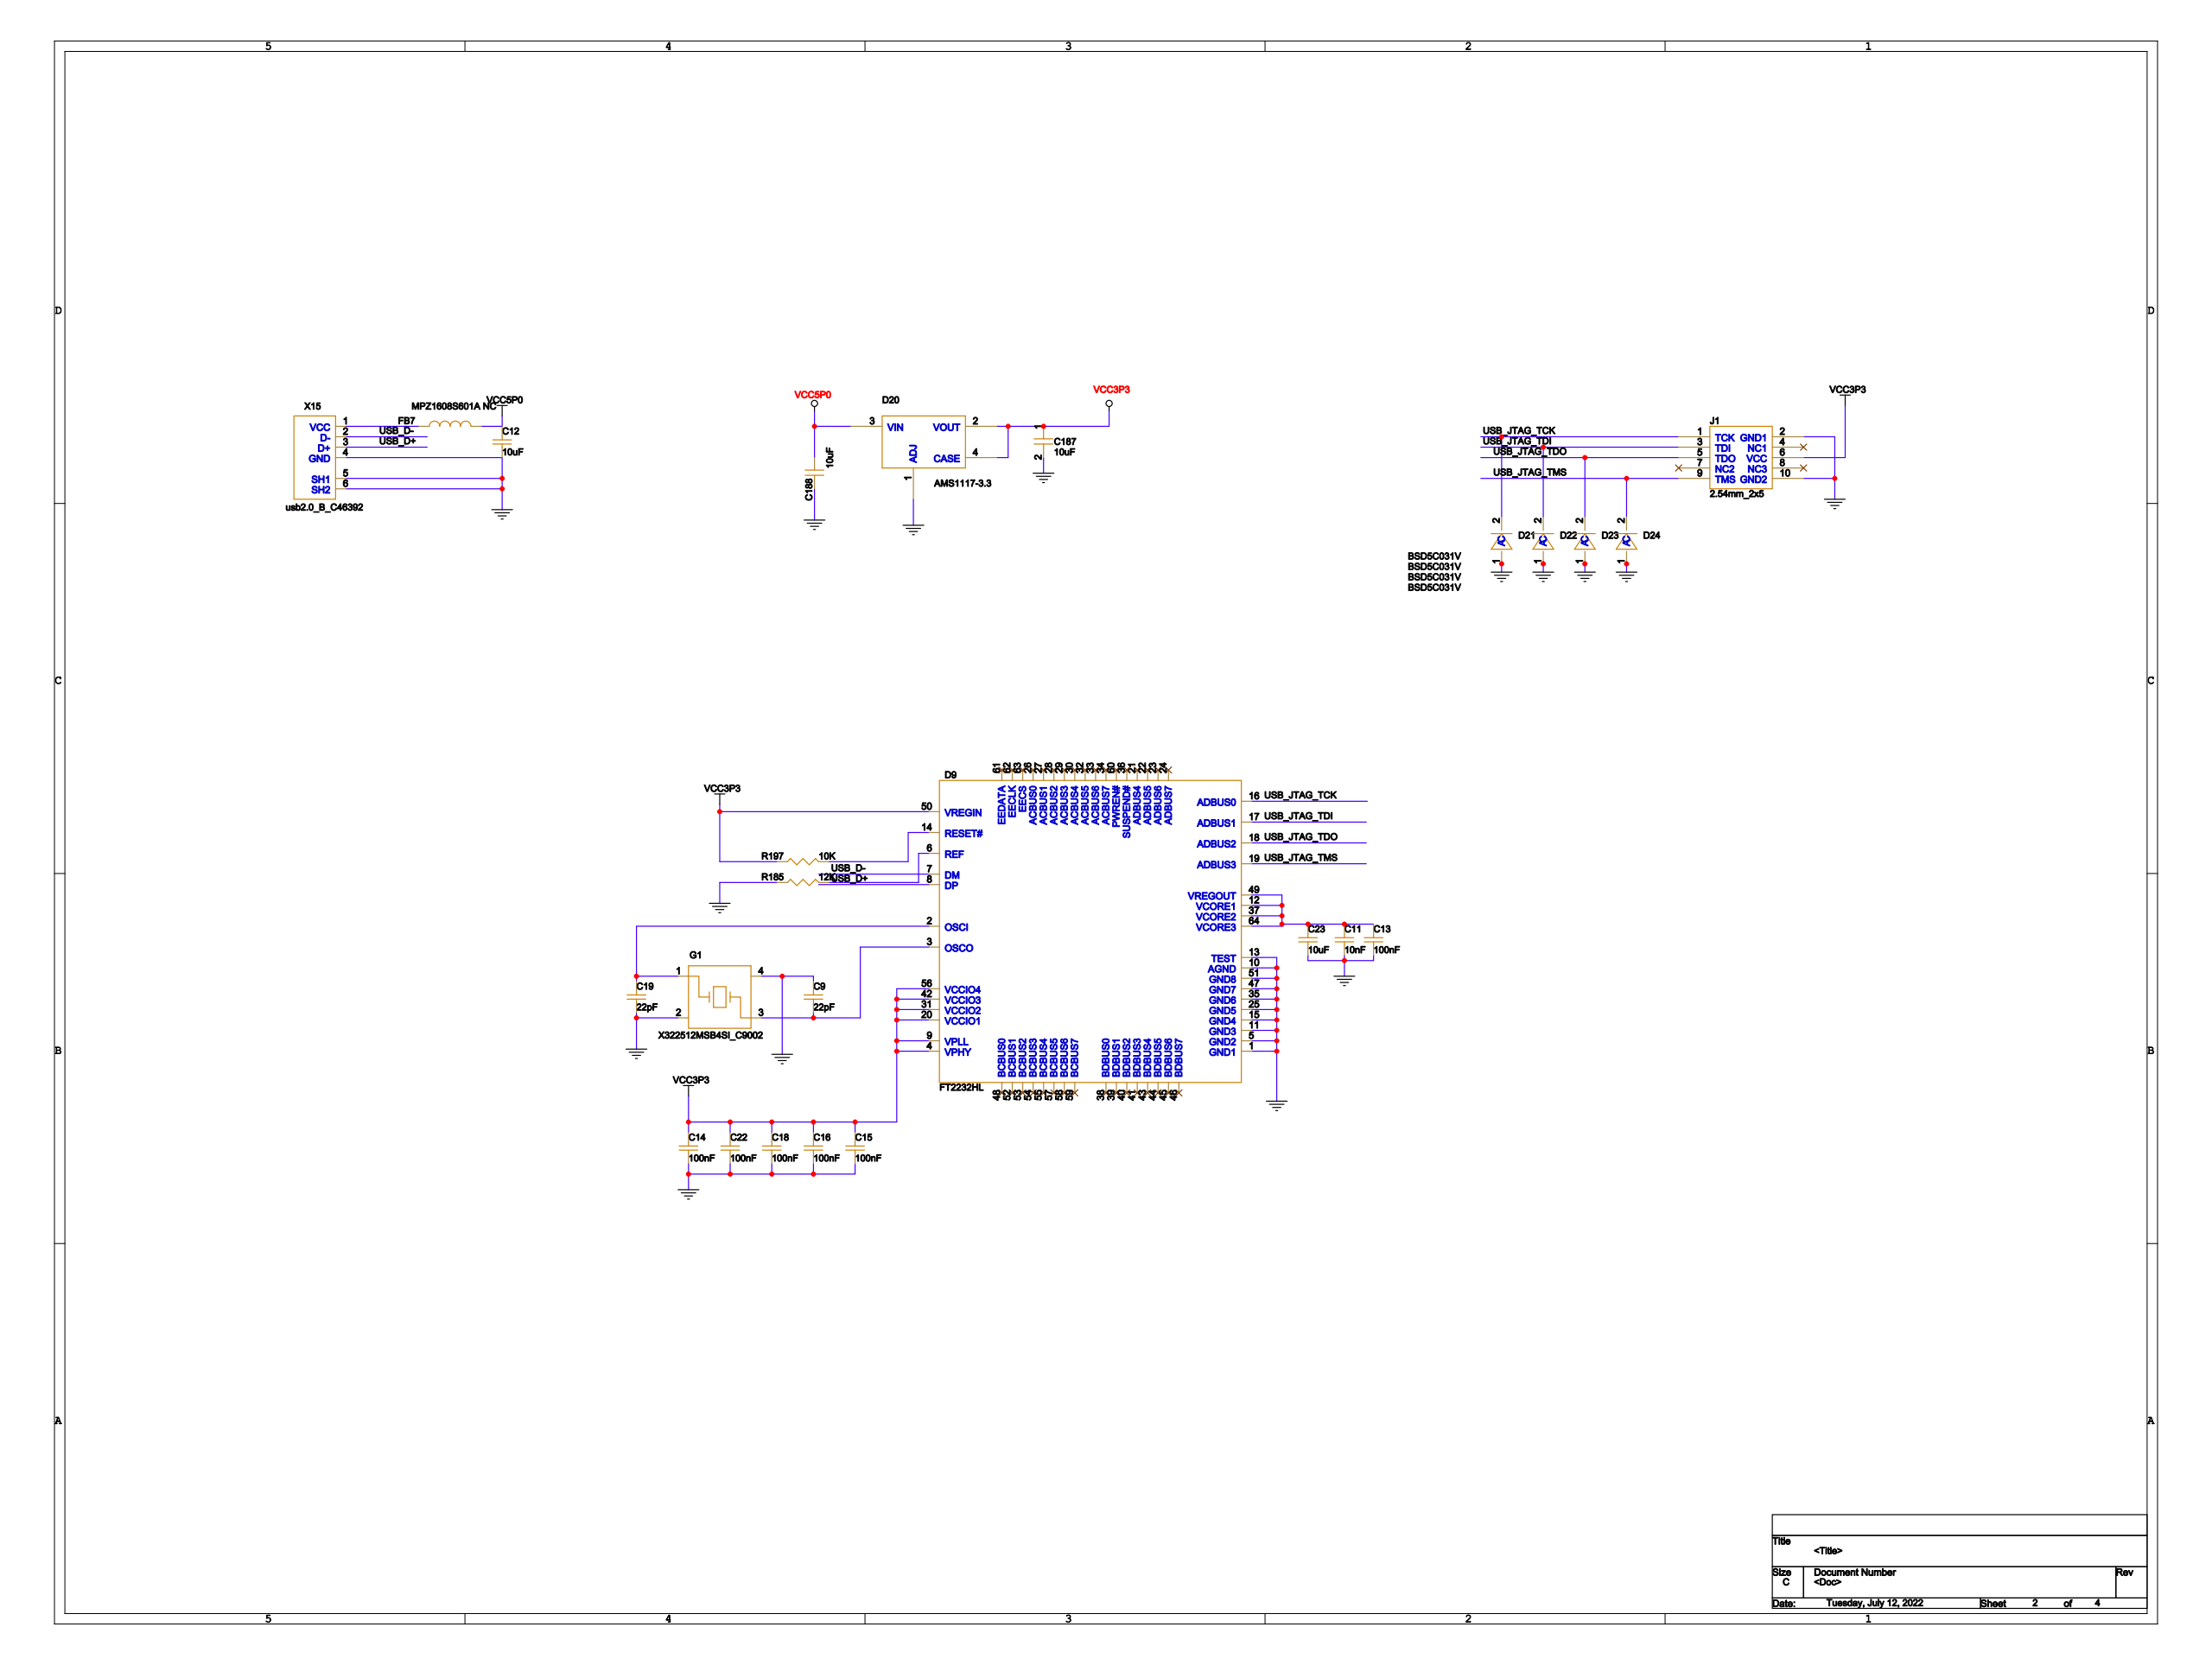Circuit board | Cadence Allegro | 25 parts | 15 nets
Bill of materials:
SYM_NAME,COMP_DEVICE_TYPE,COMP_VALUE,COMP_TOL,COMP_CLASS,REFDES
SMC0603,CAPV_SMC0603_22PF,22pF,,IC,C9
SMC0603,CAPV_SMC0603_10NF,10nF,,IC,C11
C0805,CAPV_C0805_10UF,10uF,,IC,C12
SMC0603,CAPV_SMC0603_100NF,100nF,,IC,C13
SMC0603,CAPV_SMC0603_100NF,100nF,,IC,C14
SMC0603,CAPV_SMC0603_100NF,100nF,,IC,C15
SMC0603,CAPV_SMC0603_100NF,100nF,,IC,C16
SMC0603,CAPV_SMC0603_100NF,100nF,,IC,C18
SMC0603,CAPV_SMC0603_22PF,22pF,,IC,C19
SMC0603,CAPV_SMC0603_100NF,100nF,,IC,C22
C0805,CAPV_C0805_10UF,10uF,,IC,C23
C0805,CAPACITOR NON-POL_0_C0805_10UF,10uF,,IC,C187
C0805,CAP NP_C0805_10UF,10uF,,IC,C188
LQFP64_D12_E12_P0R5,FT2232HL_0_LQFP64_D12_E12_P0R5_,FT2232HL,,IC,D9
SOT-223,BA05ST/TO_2_SOT-223_AMS1117-3.3,AMS1117-3.3,,IC,D20
SOD-523_L1_2-W0_8-LS1_6-BI,DIODE_0_SOD-523_L1_2-W0_8-LS1_6,BSD5C031V,,IC,D21
SOD-523_L1_2-W0_8-LS1_6-BI,DIODE_0_SOD-523_L1_2-W0_8-LS1_6,BSD5C031V,,IC,D22
SOD-523_L1_2-W0_8-LS1_6-BI,DIODE_0_SOD-523_L1_2-W0_8-LS1_6,BSD5C031V,,IC,D23
SOD-523_L1_2-W0_8-LS1_6-BI,DIODE_0_SOD-523_L1_2-W0_8-LS1_6,BSD5C031V,,IC,D24
FB0603,INDUCTOR_H_FB0603_MPZ1608S601A,MPZ1608S601A NC,,IC,FB7
3225,CRYSTAL13_3225_IC_X322525MSB4SI,X322525MSB4SI_C13740,,IC,G1
IDC-TH_10P-P2_54-H-R2-C5-S2_54,CON4X2_0_IDC-TH_10P-P2_54-H-R2-,2.54mm_2x5,,IC,J1
R0603,R_R0603_12K,12K,,IC,R185
R0603,R_R0603_10K,10K,,IC,R197
USB-B_TH_BF90,MINI-USB-B_0_USB-B_TH_BF90_USB2,usb2.0_B_C46392,,IC,X15
Netlist (net: part-pin ...):
GND: C9-1 C11-2 C12-2 C13-2 C14-2 C15-2 C16-2 C18-2 C19-2 C22-2 C23-2 C187-2 C188-2 D9-1 D9-5 D9-10 D9-11 D9-13 D9-15 D9-25 D9-35 D9-47 D9-51 D20-1 D21-1 D22-1 D23-1 D24-1 G1-2 G1-4 J1-2 J1-10 R185-1 X15-4 X15-5 X15-6
USB_JTAG_TCK: D9-16 D21-2 J1-1
USB_JTAG_TDI: D9-17 D22-2 J1-3
USB_JTAG_TDO: D9-18 D23-2 J1-5
USB_JTAG_TMS: D9-19 D24-2 J1-9
VCC3P3: C14-1 C15-1 C16-1 C18-1 C22-1 C187-1 D9-4 D9-9 D9-20 D9-31 D9-42 D9-50 D9-56 D20-2 D20-4 J1-6 R197-1
USB_D+: D9-8 X15-3
USB_D-: D9-7 X15-2
N2533643: FB7-1 X15-1
VCC5P0: C12-1 C188-1 D20-3 FB7-2
N2533019: C19-1 D9-2 G1-1
N2533051: C9-2 D9-3 G1-3
N2533401: C11-1 C13-1 C23-1 D9-12 D9-37 D9-49 D9-64
N2532991: D9-6 R185-2
N2532947: D9-14 R197-2